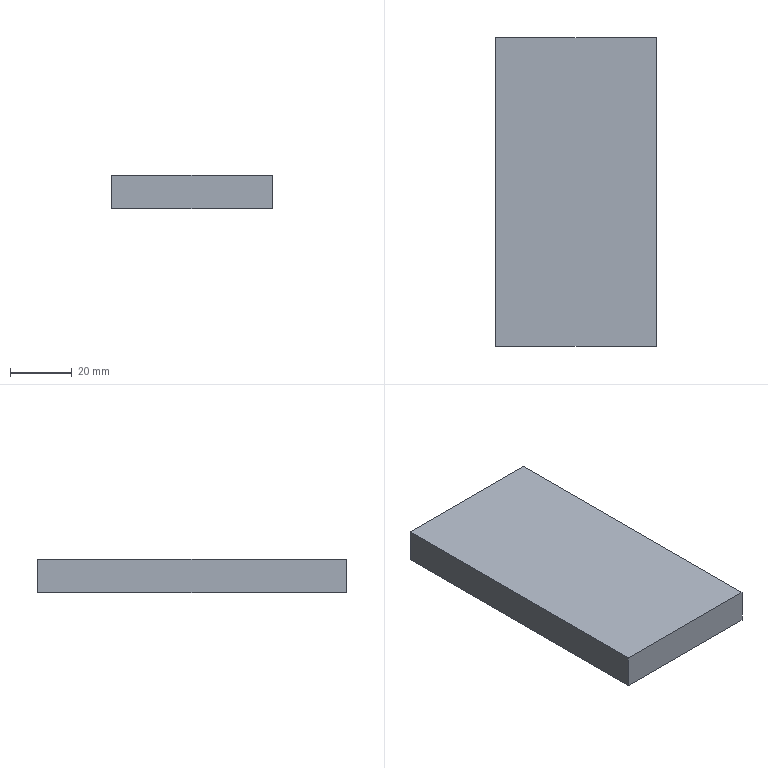Part | STEP file | Cut-Extrude 31[3] | 1 solid | 6 faces | box 52 x 100 x 11 mm | volume 57200 mm3 | plane 6
STEP:
#1=CARTESIAN_POINT('',(-830.738,-321.736,2984.5));
#2=VERTEX_POINT('',#1);
#3=CARTESIAN_POINT('',(-830.738,-421.736,2984.5));
#4=VERTEX_POINT('',#3);
#5=CARTESIAN_POINT('',(-830.738,-321.736,2984.5));
#6=DIRECTION('',(0.,-1.,0.));
#7=VECTOR('',#6,1000.);
#8=LINE('',#5,#7);
#9=EDGE_CURVE('',#2,#4,#8,.T.);
#10=ORIENTED_EDGE('',*,*,#9,.T.);
#11=CARTESIAN_POINT('',(-778.738,-421.736,2984.5));
#12=VERTEX_POINT('',#11);
#13=CARTESIAN_POINT('',(-830.738,-421.736,2984.5));
#14=DIRECTION('',(1.,0.,0.));
#15=VECTOR('',#14,1000.);
#16=LINE('',#13,#15);
#17=EDGE_CURVE('',#4,#12,#16,.T.);
#18=ORIENTED_EDGE('',*,*,#17,.T.);
#19=CARTESIAN_POINT('',(-778.738,-321.736,2984.5));
#20=VERTEX_POINT('',#19);
#21=CARTESIAN_POINT('',(-778.738,-321.736,2984.5));
#22=DIRECTION('',(0.,1.,0.));
#23=VECTOR('',#22,1000.);
#24=LINE('',#21,#23);
#25=EDGE_CURVE('',#12,#20,#24,.T.);
#26=ORIENTED_EDGE('',*,*,#25,.T.);
#27=CARTESIAN_POINT('',(-830.738,-321.736,2984.5));
#28=DIRECTION('',(-1.,0.,0.));
#29=VECTOR('',#28,1000.);
#30=LINE('',#27,#29);
#31=EDGE_CURVE('',#20,#2,#30,.T.);
#32=ORIENTED_EDGE('',*,*,#31,.T.);
#33=EDGE_LOOP('',(#10,#18,#26,#32));
#34=FACE_OUTER_BOUND('',#33,.T.);
#35=CARTESIAN_POINT('',(-748.738,-924.736,2984.5));
#36=DIRECTION('',(0.,0.,1.));
#37=DIRECTION('',(-1.,0.,0.));
#38=AXIS2_PLACEMENT_3D('',#35,#36,#37);
#39=PLANE('',#38);
#40=ADVANCED_FACE('',(#34),#39,.T.);
#41=CARTESIAN_POINT('',(-778.738,-321.736,2973.5));
#42=VERTEX_POINT('',#41);
#43=CARTESIAN_POINT('',(-830.738,-321.736,2973.5));
#44=VERTEX_POINT('',#43);
#45=CARTESIAN_POINT('',(-830.738,-321.736,2973.5));
#46=DIRECTION('',(-1.,0.,0.));
#47=VECTOR('',#46,1000.);
#48=LINE('',#45,#47);
#49=EDGE_CURVE('',#42,#44,#48,.T.);
#50=ORIENTED_EDGE('',*,*,#49,.T.);
#51=CARTESIAN_POINT('',(-830.738,-321.736,2984.5));
#52=DIRECTION('',(0.,0.,-1.));
#53=VECTOR('',#52,1000.);
#54=LINE('',#51,#53);
#55=EDGE_CURVE('',#2,#44,#54,.T.);
#56=ORIENTED_EDGE('',*,*,#55,.F.);
#57=ORIENTED_EDGE('',*,*,#31,.F.);
#58=CARTESIAN_POINT('',(-778.738,-321.736,2984.5));
#59=DIRECTION('',(0.,0.,-1.));
#60=VECTOR('',#59,1000.);
#61=LINE('',#58,#60);
#62=EDGE_CURVE('',#20,#42,#61,.T.);
#63=ORIENTED_EDGE('',*,*,#62,.T.);
#64=EDGE_LOOP('',(#50,#56,#57,#63));
#65=FACE_OUTER_BOUND('',#64,.T.);
#66=CARTESIAN_POINT('',(-830.738,-321.736,2984.5));
#67=DIRECTION('',(0.,-1.,0.));
#68=DIRECTION('',(0.,0.,1.));
#69=AXIS2_PLACEMENT_3D('',#66,#67,#68);
#70=PLANE('',#69);
#71=ADVANCED_FACE('',(#65),#70,.F.);
#72=CARTESIAN_POINT('',(-778.738,-421.736,2973.5));
#73=VERTEX_POINT('',#72);
#74=CARTESIAN_POINT('',(-778.738,-321.736,2973.5));
#75=DIRECTION('',(0.,1.,0.));
#76=VECTOR('',#75,1000.);
#77=LINE('',#74,#76);
#78=EDGE_CURVE('',#73,#42,#77,.T.);
#79=ORIENTED_EDGE('',*,*,#78,.T.);
#80=ORIENTED_EDGE('',*,*,#62,.F.);
#81=ORIENTED_EDGE('',*,*,#25,.F.);
#82=CARTESIAN_POINT('',(-778.738,-421.736,2984.5));
#83=DIRECTION('',(0.,0.,-1.));
#84=VECTOR('',#83,1000.);
#85=LINE('',#82,#84);
#86=EDGE_CURVE('',#12,#73,#85,.T.);
#87=ORIENTED_EDGE('',*,*,#86,.T.);
#88=EDGE_LOOP('',(#79,#80,#81,#87));
#89=FACE_OUTER_BOUND('',#88,.T.);
#90=CARTESIAN_POINT('',(-778.738,-321.736,2984.5));
#91=DIRECTION('',(-1.,0.,0.));
#92=DIRECTION('',(0.,1.,0.));
#93=AXIS2_PLACEMENT_3D('',#90,#91,#92);
#94=PLANE('',#93);
#95=ADVANCED_FACE('',(#89),#94,.F.);
#96=CARTESIAN_POINT('',(-830.738,-421.736,2973.5));
#97=VERTEX_POINT('',#96);
#98=CARTESIAN_POINT('',(-830.738,-421.736,2973.5));
#99=DIRECTION('',(1.,0.,0.));
#100=VECTOR('',#99,1000.);
#101=LINE('',#98,#100);
#102=EDGE_CURVE('',#97,#73,#101,.T.);
#103=ORIENTED_EDGE('',*,*,#102,.T.);
#104=ORIENTED_EDGE('',*,*,#86,.F.);
#105=ORIENTED_EDGE('',*,*,#17,.F.);
#106=CARTESIAN_POINT('',(-830.738,-421.736,2984.5));
#107=DIRECTION('',(0.,0.,-1.));
#108=VECTOR('',#107,1000.);
#109=LINE('',#106,#108);
#110=EDGE_CURVE('',#4,#97,#109,.T.);
#111=ORIENTED_EDGE('',*,*,#110,.T.);
#112=EDGE_LOOP('',(#103,#104,#105,#111));
#113=FACE_OUTER_BOUND('',#112,.T.);
#114=CARTESIAN_POINT('',(-830.738,-421.736,2984.5));
#115=DIRECTION('',(0.,1.,0.));
#116=DIRECTION('',(0.,0.,-1.));
#117=AXIS2_PLACEMENT_3D('',#114,#115,#116);
#118=PLANE('',#117);
#119=ADVANCED_FACE('',(#113),#118,.F.);
#120=CARTESIAN_POINT('',(-830.738,-321.736,2973.5));
#121=DIRECTION('',(0.,-1.,0.));
#122=VECTOR('',#121,1000.);
#123=LINE('',#120,#122);
#124=EDGE_CURVE('',#44,#97,#123,.T.);
#125=ORIENTED_EDGE('',*,*,#124,.T.);
#126=ORIENTED_EDGE('',*,*,#110,.F.);
#127=ORIENTED_EDGE('',*,*,#9,.F.);
#128=ORIENTED_EDGE('',*,*,#55,.T.);
#129=EDGE_LOOP('',(#125,#126,#127,#128));
#130=FACE_OUTER_BOUND('',#129,.T.);
#131=CARTESIAN_POINT('',(-830.738,-321.736,2984.5));
#132=DIRECTION('',(1.,0.,0.));
#133=DIRECTION('',(0.,-1.,0.));
#134=AXIS2_PLACEMENT_3D('',#131,#132,#133);
#135=PLANE('',#134);
#136=ADVANCED_FACE('',(#130),#135,.F.);
#137=ORIENTED_EDGE('',*,*,#124,.F.);
#138=ORIENTED_EDGE('',*,*,#49,.F.);
#139=ORIENTED_EDGE('',*,*,#78,.F.);
#140=ORIENTED_EDGE('',*,*,#102,.F.);
#141=EDGE_LOOP('',(#137,#138,#139,#140));
#142=FACE_OUTER_BOUND('',#141,.T.);
#143=CARTESIAN_POINT('',(-748.738,-924.736,2973.5));
#144=DIRECTION('',(0.,0.,-1.));
#145=DIRECTION('',(1.,0.,0.));
#146=AXIS2_PLACEMENT_3D('',#143,#144,#145);
#147=PLANE('',#146);
#148=ADVANCED_FACE('',(#142),#147,.T.);
#149=CLOSED_SHELL('',(#40,#71,#95,#119,#136,#148));
#150=MANIFOLD_SOLID_BREP('',#149);
#151=CARTESIAN_POINT('',(0.,0.,0.));
#152=DIRECTION('',(0.,0.,1.));
#153=DIRECTION('',(1.,0.,0.));
#154=AXIS2_PLACEMENT_3D('',#151,#152,#153);
#155=(LENGTH_UNIT()NAMED_UNIT(*)SI_UNIT(.MILLI.,.METRE.));
#156=UNCERTAINTY_MEASURE_WITH_UNIT(LENGTH_MEASURE(0.00001),#155,'','');
#157=(NAMED_UNIT(*)PLANE_ANGLE_UNIT()SI_UNIT($,.RADIAN.));
#158=(NAMED_UNIT(*)SI_UNIT($,.STERADIAN.)SOLID_ANGLE_UNIT());
#159=(GEOMETRIC_REPRESENTATION_CONTEXT(3)GLOBAL_UNCERTAINTY_ASSIGNED_CONTEXT((#156))GLOBAL_UNIT_ASSIGNED_CONTEXT((#155,#157,#158))REPRESENTATION_CONTEXT('',''));
#160=ADVANCED_BREP_SHAPE_REPRESENTATION('',(#150,#154),#159);